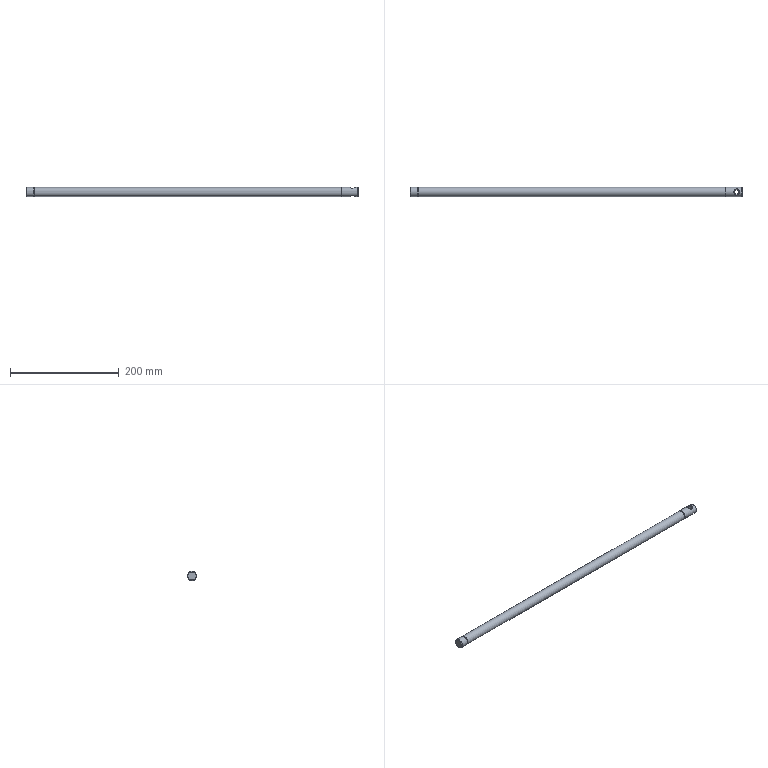Part | STEP file | Q7C0702 | 1 solid | 16 faces | box 610 x 17 x 17 mm | volume 138904 mm3 | cylinder 6 | plane 6 | cone 2 | spline 2 | commonest cylinder face diameters 17 x3 15.6 x2 8 x1